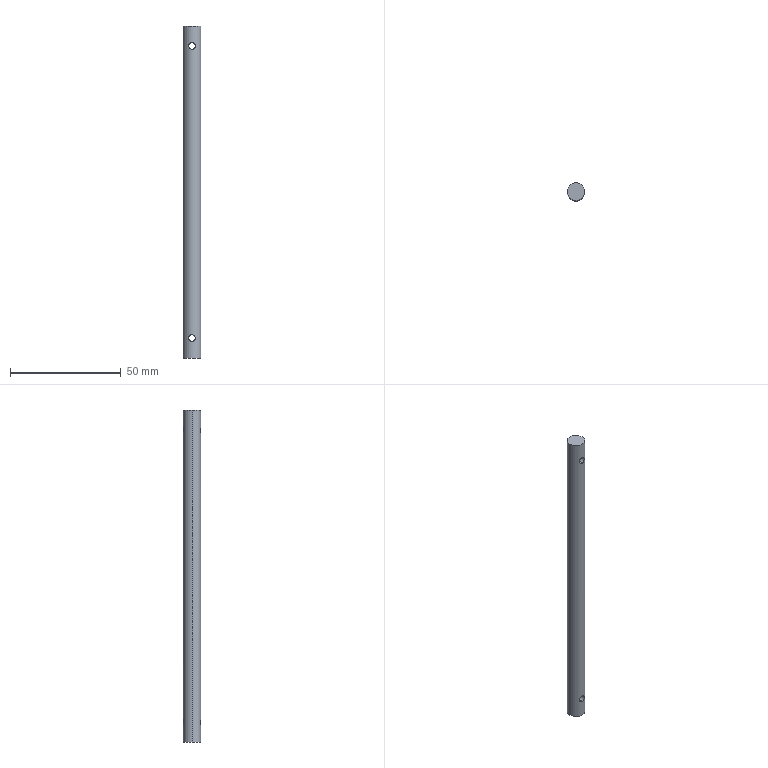Part | SolidWorks | features Extrusion 1, ICE 1 | 1 solid | 8 faces | box 8 x 8 x 150 mm | volume 7429 mm3 | cylinder 6 | plane 2 | commonest cylinder face diameters 3 x4 8 x2
STEP:
#1=CARTESIAN_POINT('',(0.,-4.,64.5));
#2=VERTEX_POINT('',#1);
#3=CARTESIAN_POINT('',(0.,-4.,67.5));
#4=VERTEX_POINT('',#3);
#5=CARTESIAN_POINT('',(0.,-4.,64.5));
#6=CARTESIAN_POINT('',(-0.1971,-4.,64.5));
#7=CARTESIAN_POINT('',(-0.396,-3.985,64.54));
#8=CARTESIAN_POINT('',(-0.6679,-3.945,64.653));
#9=CARTESIAN_POINT('',(-0.7555,-3.929,64.7));
#10=CARTESIAN_POINT('',(-0.917,-3.894,64.809));
#11=CARTESIAN_POINT('',(-0.9921,-3.876,64.871));
#12=CARTESIAN_POINT('',(-1.2,-3.818,65.079));
#13=CARTESIAN_POINT('',(-1.309,-3.78,65.242));
#14=CARTESIAN_POINT('',(-1.423,-3.739,65.515));
#15=CARTESIAN_POINT('',(-1.451,-3.727,65.608));
#16=CARTESIAN_POINT('',(-1.49,-3.712,65.801));
#17=CARTESIAN_POINT('',(-1.5,-3.708,65.902));
#18=CARTESIAN_POINT('',(-1.5,-3.708,66.198));
#19=CARTESIAN_POINT('',(-1.46,-3.725,66.397));
#20=CARTESIAN_POINT('',(-1.309,-3.781,66.758));
#21=CARTESIAN_POINT('',(-1.198,-3.819,66.923));
#22=CARTESIAN_POINT('',(-0.9915,-3.876,67.13));
#23=CARTESIAN_POINT('',(-0.9151,-3.895,67.193));
#24=CARTESIAN_POINT('',(-0.7535,-3.929,67.301));
#25=CARTESIAN_POINT('',(-0.6678,-3.945,67.347));
#26=CARTESIAN_POINT('',(-0.3945,-3.985,67.461));
#27=CARTESIAN_POINT('',(-0.2002,-4.,67.5));
#28=CARTESIAN_POINT('',(0.,-4.,67.5));
#29=B_SPLINE_CURVE_WITH_KNOTS('',3,(#5,#6,#7,#8,#9,#10,#11,#12,#13,#14,#15,#16,#17,#18,#19,#20,#21,#22,#23,#24,#25,#26,#27,#28),.UNSPECIFIED.,.F.,.F.,(4,2,2,2,2,2,2,2,2,2,2,4),(0.004733,0.005325,0.005621,0.005916,0.006508,0.006804,0.0071,0.007691,0.008283,0.008578,0.008874,0.009466),.UNSPECIFIED.);
#30=EDGE_CURVE('',#2,#4,#29,.T.);
#31=ORIENTED_EDGE('',*,*,#30,.F.);
#32=CARTESIAN_POINT('',(0.,4.,64.5));
#33=VERTEX_POINT('',#32);
#34=CARTESIAN_POINT('',(0.,-5.,64.5));
#35=DIRECTION('',(0.,1.,0.));
#36=VECTOR('',#35,1000.);
#37=LINE('',#34,#36);
#38=EDGE_CURVE('',#2,#33,#37,.T.);
#39=ORIENTED_EDGE('',*,*,#38,.T.);
#40=CARTESIAN_POINT('',(0.,4.,67.5));
#41=VERTEX_POINT('',#40);
#42=CARTESIAN_POINT('',(0.,4.,67.5));
#43=CARTESIAN_POINT('',(-0.1001,4.,67.5));
#44=CARTESIAN_POINT('',(-0.1983,3.996,67.49));
#45=CARTESIAN_POINT('',(-0.3914,3.982,67.451));
#46=CARTESIAN_POINT('',(-0.4871,3.971,67.422));
#47=CARTESIAN_POINT('',(-0.7591,3.932,67.309));
#48=CARTESIAN_POINT('',(-0.9243,3.894,67.197));
#49=CARTESIAN_POINT('',(-1.198,3.819,66.923));
#50=CARTESIAN_POINT('',(-1.309,3.78,66.757));
#51=CARTESIAN_POINT('',(-1.422,3.739,66.487));
#52=CARTESIAN_POINT('',(-1.451,3.727,66.392));
#53=CARTESIAN_POINT('',(-1.49,3.712,66.198));
#54=CARTESIAN_POINT('',(-1.5,3.708,66.1));
#55=CARTESIAN_POINT('',(-1.5,3.708,65.902));
#56=CARTESIAN_POINT('',(-1.49,3.712,65.802));
#57=CARTESIAN_POINT('',(-1.451,3.727,65.608));
#58=CARTESIAN_POINT('',(-1.423,3.739,65.514));
#59=CARTESIAN_POINT('',(-1.346,3.767,65.332));
#60=CARTESIAN_POINT('',(-1.3,3.783,65.246));
#61=CARTESIAN_POINT('',(-1.192,3.819,65.084));
#62=CARTESIAN_POINT('',(-1.129,3.838,65.008));
#63=CARTESIAN_POINT('',(-0.9914,3.876,64.87));
#64=CARTESIAN_POINT('',(-0.9166,3.894,64.809));
#65=CARTESIAN_POINT('',(-0.7545,3.929,64.7));
#66=CARTESIAN_POINT('',(-0.6669,3.945,64.653));
#67=CARTESIAN_POINT('',(-0.3963,3.984,64.54));
#68=CARTESIAN_POINT('',(-0.1972,4.,64.5));
#69=CARTESIAN_POINT('',(0.,4.,64.5));
#70=B_SPLINE_CURVE_WITH_KNOTS('',3,(#42,#43,#44,#45,#46,#47,#48,#49,#50,#51,#52,#53,#54,#55,#56,#57,#58,#59,#60,#61,#62,#63,#64,#65,#66,#67,#68,#69),.UNSPECIFIED.,.F.,.F.,(4,2,2,2,2,2,2,2,2,2,2,2,2,4),(0.,0.0002958,0.0005917,0.001183,0.001775,0.002071,0.002367,0.002663,0.002958,0.003254,0.00355,0.003846,0.004142,0.004733),.UNSPECIFIED.);
#71=EDGE_CURVE('',#41,#33,#70,.T.);
#72=ORIENTED_EDGE('',*,*,#71,.F.);
#73=CARTESIAN_POINT('',(0.,-5.,67.5));
#74=DIRECTION('',(0.,1.,0.));
#75=VECTOR('',#74,1000.);
#76=LINE('',#73,#75);
#77=EDGE_CURVE('',#4,#41,#76,.T.);
#78=ORIENTED_EDGE('',*,*,#77,.F.);
#79=EDGE_LOOP('',(#31,#39,#72,#78));
#80=FACE_OUTER_BOUND('',#79,.T.);
#81=CARTESIAN_POINT('',(0.,-5.,66.));
#82=DIRECTION('',(0.,1.,0.));
#83=DIRECTION('',(0.,0.,1.));
#84=AXIS2_PLACEMENT_3D('',#81,#82,#83);
#85=CYLINDRICAL_SURFACE('',#84,1.5);
#86=ADVANCED_FACE('',(#80),#85,.F.);
#87=CARTESIAN_POINT('',(0.,-4.,-67.5));
#88=VERTEX_POINT('',#87);
#89=CARTESIAN_POINT('',(0.,-4.,-64.5));
#90=VERTEX_POINT('',#89);
#91=CARTESIAN_POINT('',(0.,-4.,-67.5));
#92=CARTESIAN_POINT('',(-0.1971,-4.,-67.5));
#93=CARTESIAN_POINT('',(-0.396,-3.985,-67.46));
#94=CARTESIAN_POINT('',(-0.6679,-3.945,-67.347));
#95=CARTESIAN_POINT('',(-0.7555,-3.929,-67.3));
#96=CARTESIAN_POINT('',(-0.917,-3.894,-67.191));
#97=CARTESIAN_POINT('',(-0.9921,-3.876,-67.129));
#98=CARTESIAN_POINT('',(-1.2,-3.818,-66.921));
#99=CARTESIAN_POINT('',(-1.309,-3.78,-66.758));
#100=CARTESIAN_POINT('',(-1.423,-3.739,-66.485));
#101=CARTESIAN_POINT('',(-1.451,-3.727,-66.392));
#102=CARTESIAN_POINT('',(-1.49,-3.712,-66.199));
#103=CARTESIAN_POINT('',(-1.5,-3.708,-66.098));
#104=CARTESIAN_POINT('',(-1.5,-3.708,-65.802));
#105=CARTESIAN_POINT('',(-1.46,-3.725,-65.603));
#106=CARTESIAN_POINT('',(-1.309,-3.781,-65.242));
#107=CARTESIAN_POINT('',(-1.198,-3.819,-65.077));
#108=CARTESIAN_POINT('',(-0.9915,-3.876,-64.87));
#109=CARTESIAN_POINT('',(-0.9151,-3.895,-64.807));
#110=CARTESIAN_POINT('',(-0.7535,-3.929,-64.699));
#111=CARTESIAN_POINT('',(-0.6678,-3.945,-64.653));
#112=CARTESIAN_POINT('',(-0.3945,-3.985,-64.539));
#113=CARTESIAN_POINT('',(-0.2002,-4.,-64.5));
#114=CARTESIAN_POINT('',(0.,-4.,-64.5));
#115=B_SPLINE_CURVE_WITH_KNOTS('',3,(#91,#92,#93,#94,#95,#96,#97,#98,#99,#100,#101,#102,#103,#104,#105,#106,#107,#108,#109,#110,#111,#112,#113,#114),.UNSPECIFIED.,.F.,.F.,(4,2,2,2,2,2,2,2,2,2,2,4),(0.004733,0.005325,0.005621,0.005916,0.006508,0.006804,0.0071,0.007691,0.008283,0.008578,0.008874,0.009466),.UNSPECIFIED.);
#116=EDGE_CURVE('',#88,#90,#115,.T.);
#117=ORIENTED_EDGE('',*,*,#116,.F.);
#118=CARTESIAN_POINT('',(0.,4.,-67.5));
#119=VERTEX_POINT('',#118);
#120=CARTESIAN_POINT('',(0.,-5.,-67.5));
#121=DIRECTION('',(0.,1.,0.));
#122=VECTOR('',#121,1000.);
#123=LINE('',#120,#122);
#124=EDGE_CURVE('',#88,#119,#123,.T.);
#125=ORIENTED_EDGE('',*,*,#124,.T.);
#126=CARTESIAN_POINT('',(0.,4.,-64.5));
#127=VERTEX_POINT('',#126);
#128=CARTESIAN_POINT('',(0.,4.,-64.5));
#129=CARTESIAN_POINT('',(-0.1001,4.,-64.5));
#130=CARTESIAN_POINT('',(-0.1983,3.996,-64.51));
#131=CARTESIAN_POINT('',(-0.3914,3.982,-64.549));
#132=CARTESIAN_POINT('',(-0.4871,3.971,-64.578));
#133=CARTESIAN_POINT('',(-0.7591,3.932,-64.691));
#134=CARTESIAN_POINT('',(-0.9243,3.894,-64.803));
#135=CARTESIAN_POINT('',(-1.198,3.819,-65.077));
#136=CARTESIAN_POINT('',(-1.309,3.78,-65.243));
#137=CARTESIAN_POINT('',(-1.422,3.739,-65.513));
#138=CARTESIAN_POINT('',(-1.451,3.727,-65.608));
#139=CARTESIAN_POINT('',(-1.49,3.712,-65.802));
#140=CARTESIAN_POINT('',(-1.5,3.708,-65.9));
#141=CARTESIAN_POINT('',(-1.5,3.708,-66.098));
#142=CARTESIAN_POINT('',(-1.49,3.712,-66.198));
#143=CARTESIAN_POINT('',(-1.451,3.727,-66.392));
#144=CARTESIAN_POINT('',(-1.423,3.739,-66.486));
#145=CARTESIAN_POINT('',(-1.346,3.767,-66.668));
#146=CARTESIAN_POINT('',(-1.3,3.783,-66.754));
#147=CARTESIAN_POINT('',(-1.192,3.819,-66.916));
#148=CARTESIAN_POINT('',(-1.129,3.838,-66.992));
#149=CARTESIAN_POINT('',(-0.9914,3.876,-67.13));
#150=CARTESIAN_POINT('',(-0.9166,3.894,-67.191));
#151=CARTESIAN_POINT('',(-0.7545,3.929,-67.3));
#152=CARTESIAN_POINT('',(-0.6669,3.945,-67.347));
#153=CARTESIAN_POINT('',(-0.3963,3.984,-67.46));
#154=CARTESIAN_POINT('',(-0.1972,4.,-67.5));
#155=CARTESIAN_POINT('',(0.,4.,-67.5));
#156=B_SPLINE_CURVE_WITH_KNOTS('',3,(#128,#129,#130,#131,#132,#133,#134,#135,#136,#137,#138,#139,#140,#141,#142,#143,#144,#145,#146,#147,#148,#149,#150,#151,#152,#153,#154,#155),.UNSPECIFIED.,.F.,.F.,(4,2,2,2,2,2,2,2,2,2,2,2,2,4),(0.,0.0002958,0.0005917,0.001183,0.001775,0.002071,0.002367,0.002663,0.002958,0.003254,0.00355,0.003846,0.004142,0.004733),.UNSPECIFIED.);
#157=EDGE_CURVE('',#127,#119,#156,.T.);
#158=ORIENTED_EDGE('',*,*,#157,.F.);
#159=CARTESIAN_POINT('',(0.,-5.,-64.5));
#160=DIRECTION('',(0.,1.,0.));
#161=VECTOR('',#160,1000.);
#162=LINE('',#159,#161);
#163=EDGE_CURVE('',#90,#127,#162,.T.);
#164=ORIENTED_EDGE('',*,*,#163,.F.);
#165=EDGE_LOOP('',(#117,#125,#158,#164));
#166=FACE_OUTER_BOUND('',#165,.T.);
#167=CARTESIAN_POINT('',(0.,-5.,-66.));
#168=DIRECTION('',(0.,1.,0.));
#169=DIRECTION('',(0.,0.,1.));
#170=AXIS2_PLACEMENT_3D('',#167,#168,#169);
#171=CYLINDRICAL_SURFACE('',#170,1.5);
#172=ADVANCED_FACE('',(#166),#171,.F.);
#173=ORIENTED_EDGE('',*,*,#157,.T.);
#174=CARTESIAN_POINT('',(0.,4.,-67.5));
#175=CARTESIAN_POINT('',(0.1971,4.,-67.5));
#176=CARTESIAN_POINT('',(0.396,3.985,-67.46));
#177=CARTESIAN_POINT('',(0.6679,3.945,-67.347));
#178=CARTESIAN_POINT('',(0.7555,3.929,-67.3));
#179=CARTESIAN_POINT('',(0.917,3.894,-67.191));
#180=CARTESIAN_POINT('',(0.9921,3.876,-67.129));
#181=CARTESIAN_POINT('',(1.2,3.818,-66.921));
#182=CARTESIAN_POINT('',(1.309,3.78,-66.758));
#183=CARTESIAN_POINT('',(1.423,3.739,-66.485));
#184=CARTESIAN_POINT('',(1.451,3.727,-66.392));
#185=CARTESIAN_POINT('',(1.49,3.712,-66.199));
#186=CARTESIAN_POINT('',(1.5,3.708,-66.098));
#187=CARTESIAN_POINT('',(1.5,3.708,-65.802));
#188=CARTESIAN_POINT('',(1.46,3.725,-65.603));
#189=CARTESIAN_POINT('',(1.309,3.781,-65.242));
#190=CARTESIAN_POINT('',(1.198,3.819,-65.077));
#191=CARTESIAN_POINT('',(0.9915,3.876,-64.87));
#192=CARTESIAN_POINT('',(0.9151,3.895,-64.807));
#193=CARTESIAN_POINT('',(0.7535,3.929,-64.699));
#194=CARTESIAN_POINT('',(0.6678,3.945,-64.653));
#195=CARTESIAN_POINT('',(0.3945,3.985,-64.539));
#196=CARTESIAN_POINT('',(0.2002,4.,-64.5));
#197=CARTESIAN_POINT('',(0.,4.,-64.5));
#198=B_SPLINE_CURVE_WITH_KNOTS('',3,(#174,#175,#176,#177,#178,#179,#180,#181,#182,#183,#184,#185,#186,#187,#188,#189,#190,#191,#192,#193,#194,#195,#196,#197),.UNSPECIFIED.,.F.,.F.,(4,2,2,2,2,2,2,2,2,2,2,4),(0.004733,0.005325,0.005621,0.005916,0.006508,0.006804,0.0071,0.007691,0.008283,0.008578,0.008874,0.009466),.UNSPECIFIED.);
#199=EDGE_CURVE('',#119,#127,#198,.T.);
#200=ORIENTED_EDGE('',*,*,#199,.T.);
#201=EDGE_LOOP('',(#173,#200));
#202=FACE_BOUND('',#201,.T.);
#203=ORIENTED_EDGE('',*,*,#71,.T.);
#204=CARTESIAN_POINT('',(0.,4.,64.5));
#205=CARTESIAN_POINT('',(0.1971,4.,64.5));
#206=CARTESIAN_POINT('',(0.396,3.985,64.54));
#207=CARTESIAN_POINT('',(0.6679,3.945,64.653));
#208=CARTESIAN_POINT('',(0.7555,3.929,64.7));
#209=CARTESIAN_POINT('',(0.917,3.894,64.809));
#210=CARTESIAN_POINT('',(0.9921,3.876,64.871));
#211=CARTESIAN_POINT('',(1.2,3.818,65.079));
#212=CARTESIAN_POINT('',(1.309,3.78,65.242));
#213=CARTESIAN_POINT('',(1.423,3.739,65.515));
#214=CARTESIAN_POINT('',(1.451,3.727,65.608));
#215=CARTESIAN_POINT('',(1.49,3.712,65.801));
#216=CARTESIAN_POINT('',(1.5,3.708,65.902));
#217=CARTESIAN_POINT('',(1.5,3.708,66.198));
#218=CARTESIAN_POINT('',(1.46,3.725,66.397));
#219=CARTESIAN_POINT('',(1.309,3.781,66.758));
#220=CARTESIAN_POINT('',(1.198,3.819,66.923));
#221=CARTESIAN_POINT('',(0.9915,3.876,67.13));
#222=CARTESIAN_POINT('',(0.9151,3.895,67.193));
#223=CARTESIAN_POINT('',(0.7535,3.929,67.301));
#224=CARTESIAN_POINT('',(0.6678,3.945,67.347));
#225=CARTESIAN_POINT('',(0.3945,3.985,67.461));
#226=CARTESIAN_POINT('',(0.2002,4.,67.5));
#227=CARTESIAN_POINT('',(0.,4.,67.5));
#228=B_SPLINE_CURVE_WITH_KNOTS('',3,(#204,#205,#206,#207,#208,#209,#210,#211,#212,#213,#214,#215,#216,#217,#218,#219,#220,#221,#222,#223,#224,#225,#226,#227),.UNSPECIFIED.,.F.,.F.,(4,2,2,2,2,2,2,2,2,2,2,4),(0.004733,0.005325,0.005621,0.005916,0.006508,0.006804,0.0071,0.007691,0.008283,0.008578,0.008874,0.009466),.UNSPECIFIED.);
#229=EDGE_CURVE('',#33,#41,#228,.T.);
#230=ORIENTED_EDGE('',*,*,#229,.T.);
#231=EDGE_LOOP('',(#203,#230));
#232=FACE_BOUND('',#231,.T.);
#233=CARTESIAN_POINT('',(4.,0.,75.));
#234=VERTEX_POINT('',#233);
#235=CARTESIAN_POINT('',(-4.,0.,75.));
#236=VERTEX_POINT('',#235);
#237=CARTESIAN_POINT('',(0.,0.,75.));
#238=DIRECTION('',(0.,0.,1.));
#239=DIRECTION('',(1.,0.,0.));
#240=AXIS2_PLACEMENT_3D('',#237,#238,#239);
#241=CIRCLE('',#240,4.);
#242=EDGE_CURVE('',#234,#236,#241,.T.);
#243=ORIENTED_EDGE('',*,*,#242,.F.);
#244=CARTESIAN_POINT('',(4.,0.,-75.));
#245=VERTEX_POINT('',#244);
#246=CARTESIAN_POINT('',(4.,0.,75.));
#247=DIRECTION('',(0.,0.,-1.));
#248=VECTOR('',#247,1000.);
#249=LINE('',#246,#248);
#250=EDGE_CURVE('',#234,#245,#249,.T.);
#251=ORIENTED_EDGE('',*,*,#250,.T.);
#252=CARTESIAN_POINT('',(-4.,0.,-75.));
#253=VERTEX_POINT('',#252);
#254=CARTESIAN_POINT('',(0.,0.,-75.));
#255=DIRECTION('',(0.,0.,1.));
#256=DIRECTION('',(1.,0.,0.));
#257=AXIS2_PLACEMENT_3D('',#254,#255,#256);
#258=CIRCLE('',#257,4.);
#259=EDGE_CURVE('',#245,#253,#258,.T.);
#260=ORIENTED_EDGE('',*,*,#259,.T.);
#261=CARTESIAN_POINT('',(-4.,0.,75.));
#262=DIRECTION('',(0.,0.,-1.));
#263=VECTOR('',#262,1000.);
#264=LINE('',#261,#263);
#265=EDGE_CURVE('',#236,#253,#264,.T.);
#266=ORIENTED_EDGE('',*,*,#265,.F.);
#267=EDGE_LOOP('',(#243,#251,#260,#266));
#268=FACE_OUTER_BOUND('',#267,.T.);
#269=CARTESIAN_POINT('',(0.,0.,75.));
#270=DIRECTION('',(0.,0.,-1.));
#271=DIRECTION('',(-1.,0.,0.));
#272=AXIS2_PLACEMENT_3D('',#269,#270,#271);
#273=CYLINDRICAL_SURFACE('',#272,4.);
#274=ADVANCED_FACE('',(#202,#232,#268),#273,.T.);
#275=ORIENTED_EDGE('',*,*,#250,.F.);
#276=CARTESIAN_POINT('',(0.,0.,75.));
#277=DIRECTION('',(0.,0.,1.));
#278=DIRECTION('',(1.,0.,0.));
#279=AXIS2_PLACEMENT_3D('',#276,#277,#278);
#280=CIRCLE('',#279,4.);
#281=EDGE_CURVE('',#236,#234,#280,.T.);
#282=ORIENTED_EDGE('',*,*,#281,.F.);
#283=ORIENTED_EDGE('',*,*,#265,.T.);
#284=CARTESIAN_POINT('',(0.,0.,-75.));
#285=DIRECTION('',(0.,0.,1.));
#286=DIRECTION('',(1.,0.,0.));
#287=AXIS2_PLACEMENT_3D('',#284,#285,#286);
#288=CIRCLE('',#287,4.);
#289=EDGE_CURVE('',#253,#245,#288,.T.);
#290=ORIENTED_EDGE('',*,*,#289,.T.);
#291=EDGE_LOOP('',(#275,#282,#283,#290));
#292=FACE_OUTER_BOUND('',#291,.T.);
#293=CARTESIAN_POINT('',(0.,-4.,67.5));
#294=CARTESIAN_POINT('',(0.1001,-4.,67.5));
#295=CARTESIAN_POINT('',(0.1983,-3.996,67.49));
#296=CARTESIAN_POINT('',(0.3914,-3.982,67.451));
#297=CARTESIAN_POINT('',(0.4871,-3.971,67.422));
#298=CARTESIAN_POINT('',(0.7591,-3.932,67.309));
#299=CARTESIAN_POINT('',(0.9243,-3.894,67.197));
#300=CARTESIAN_POINT('',(1.198,-3.819,66.923));
#301=CARTESIAN_POINT('',(1.309,-3.78,66.757));
#302=CARTESIAN_POINT('',(1.422,-3.739,66.487));
#303=CARTESIAN_POINT('',(1.451,-3.727,66.392));
#304=CARTESIAN_POINT('',(1.49,-3.712,66.198));
#305=CARTESIAN_POINT('',(1.5,-3.708,66.1));
#306=CARTESIAN_POINT('',(1.5,-3.708,65.902));
#307=CARTESIAN_POINT('',(1.49,-3.712,65.802));
#308=CARTESIAN_POINT('',(1.451,-3.727,65.608));
#309=CARTESIAN_POINT('',(1.423,-3.739,65.514));
#310=CARTESIAN_POINT('',(1.346,-3.767,65.332));
#311=CARTESIAN_POINT('',(1.3,-3.783,65.246));
#312=CARTESIAN_POINT('',(1.192,-3.819,65.084));
#313=CARTESIAN_POINT('',(1.129,-3.838,65.008));
#314=CARTESIAN_POINT('',(0.9914,-3.876,64.87));
#315=CARTESIAN_POINT('',(0.9166,-3.894,64.809));
#316=CARTESIAN_POINT('',(0.7545,-3.929,64.7));
#317=CARTESIAN_POINT('',(0.6669,-3.945,64.653));
#318=CARTESIAN_POINT('',(0.3963,-3.984,64.54));
#319=CARTESIAN_POINT('',(0.1972,-4.,64.5));
#320=CARTESIAN_POINT('',(0.,-4.,64.5));
#321=B_SPLINE_CURVE_WITH_KNOTS('',3,(#293,#294,#295,#296,#297,#298,#299,#300,#301,#302,#303,#304,#305,#306,#307,#308,#309,#310,#311,#312,#313,#314,#315,#316,#317,#318,#319,#320),.UNSPECIFIED.,.F.,.F.,(4,2,2,2,2,2,2,2,2,2,2,2,2,4),(0.,0.0002958,0.0005917,0.001183,0.001775,0.002071,0.002367,0.002663,0.002958,0.003254,0.00355,0.003846,0.004142,0.004733),.UNSPECIFIED.);
#322=EDGE_CURVE('',#4,#2,#321,.T.);
#323=ORIENTED_EDGE('',*,*,#322,.T.);
#324=ORIENTED_EDGE('',*,*,#30,.T.);
#325=EDGE_LOOP('',(#323,#324));
#326=FACE_BOUND('',#325,.T.);
#327=CARTESIAN_POINT('',(0.,-4.,-64.5));
#328=CARTESIAN_POINT('',(0.1001,-4.,-64.5));
#329=CARTESIAN_POINT('',(0.1983,-3.996,-64.51));
#330=CARTESIAN_POINT('',(0.3914,-3.982,-64.549));
#331=CARTESIAN_POINT('',(0.4871,-3.971,-64.578));
#332=CARTESIAN_POINT('',(0.7591,-3.932,-64.691));
#333=CARTESIAN_POINT('',(0.9243,-3.894,-64.803));
#334=CARTESIAN_POINT('',(1.198,-3.819,-65.077));
#335=CARTESIAN_POINT('',(1.309,-3.78,-65.243));
#336=CARTESIAN_POINT('',(1.422,-3.739,-65.513));
#337=CARTESIAN_POINT('',(1.451,-3.727,-65.608));
#338=CARTESIAN_POINT('',(1.49,-3.712,-65.802));
#339=CARTESIAN_POINT('',(1.5,-3.708,-65.9));
#340=CARTESIAN_POINT('',(1.5,-3.708,-66.098));
#341=CARTESIAN_POINT('',(1.49,-3.712,-66.198));
#342=CARTESIAN_POINT('',(1.451,-3.727,-66.392));
#343=CARTESIAN_POINT('',(1.423,-3.739,-66.486));
#344=CARTESIAN_POINT('',(1.346,-3.767,-66.668));
#345=CARTESIAN_POINT('',(1.3,-3.783,-66.754));
#346=CARTESIAN_POINT('',(1.192,-3.819,-66.916));
#347=CARTESIAN_POINT('',(1.129,-3.838,-66.992));
#348=CARTESIAN_POINT('',(0.9914,-3.876,-67.13));
#349=CARTESIAN_POINT('',(0.9166,-3.894,-67.191));
#350=CARTESIAN_POINT('',(0.7545,-3.929,-67.3));
#351=CARTESIAN_POINT('',(0.6669,-3.945,-67.347));
#352=CARTESIAN_POINT('',(0.3963,-3.984,-67.46));
#353=CARTESIAN_POINT('',(0.1972,-4.,-67.5));
#354=CARTESIAN_POINT('',(0.,-4.,-67.5));
#355=B_SPLINE_CURVE_WITH_KNOTS('',3,(#327,#328,#329,#330,#331,#332,#333,#334,#335,#336,#337,#338,#339,#340,#341,#342,#343,#344,#345,#346,#347,#348,#349,#350,#351,#352,#353,#354),.UNSPECIFIED.,.F.,.F.,(4,2,2,2,2,2,2,2,2,2,2,2,2,4),(0.,0.0002958,0.0005917,0.001183,0.001775,0.002071,0.002367,0.002663,0.002958,0.003254,0.00355,0.003846,0.004142,0.004733),.UNSPECIFIED.);
#356=EDGE_CURVE('',#90,#88,#355,.T.);
#357=ORIENTED_EDGE('',*,*,#356,.T.);
#358=ORIENTED_EDGE('',*,*,#116,.T.);
#359=EDGE_LOOP('',(#357,#358));
#360=FACE_BOUND('',#359,.T.);
#361=CARTESIAN_POINT('',(0.,0.,75.));
#362=DIRECTION('',(0.,0.,-1.));
#363=DIRECTION('',(-1.,0.,0.));
#364=AXIS2_PLACEMENT_3D('',#361,#362,#363);
#365=CYLINDRICAL_SURFACE('',#364,4.);
#366=ADVANCED_FACE('',(#292,#326,#360),#365,.T.);
#367=ORIENTED_EDGE('',*,*,#281,.T.);
#368=ORIENTED_EDGE('',*,*,#242,.T.);
#369=EDGE_LOOP('',(#367,#368));
#370=FACE_OUTER_BOUND('',#369,.T.);
#371=CARTESIAN_POINT('',(0.,0.,75.));
#372=DIRECTION('',(0.,0.,1.));
#373=DIRECTION('',(1.,0.,0.));
#374=AXIS2_PLACEMENT_3D('',#371,#372,#373);
#375=PLANE('',#374);
#376=ADVANCED_FACE('',(#370),#375,.T.);
#377=ORIENTED_EDGE('',*,*,#289,.F.);
#378=ORIENTED_EDGE('',*,*,#259,.F.);
#379=EDGE_LOOP('',(#377,#378));
#380=FACE_OUTER_BOUND('',#379,.T.);
#381=CARTESIAN_POINT('',(0.,0.,-75.));
#382=DIRECTION('',(0.,0.,1.));
#383=DIRECTION('',(1.,0.,0.));
#384=AXIS2_PLACEMENT_3D('',#381,#382,#383);
#385=PLANE('',#384);
#386=ADVANCED_FACE('',(#380),#385,.F.);
#387=ORIENTED_EDGE('',*,*,#124,.F.);
#388=ORIENTED_EDGE('',*,*,#356,.F.);
#389=ORIENTED_EDGE('',*,*,#163,.T.);
#390=ORIENTED_EDGE('',*,*,#199,.F.);
#391=EDGE_LOOP('',(#387,#388,#389,#390));
#392=FACE_OUTER_BOUND('',#391,.T.);
#393=CARTESIAN_POINT('',(0.,-5.,-66.));
#394=DIRECTION('',(0.,1.,0.));
#395=DIRECTION('',(0.,0.,1.));
#396=AXIS2_PLACEMENT_3D('',#393,#394,#395);
#397=CYLINDRICAL_SURFACE('',#396,1.5);
#398=ADVANCED_FACE('',(#392),#397,.F.);
#399=ORIENTED_EDGE('',*,*,#38,.F.);
#400=ORIENTED_EDGE('',*,*,#322,.F.);
#401=ORIENTED_EDGE('',*,*,#77,.T.);
#402=ORIENTED_EDGE('',*,*,#229,.F.);
#403=EDGE_LOOP('',(#399,#400,#401,#402));
#404=FACE_OUTER_BOUND('',#403,.T.);
#405=CARTESIAN_POINT('',(0.,-5.,66.));
#406=DIRECTION('',(0.,1.,0.));
#407=DIRECTION('',(0.,0.,1.));
#408=AXIS2_PLACEMENT_3D('',#405,#406,#407);
#409=CYLINDRICAL_SURFACE('',#408,1.5);
#410=ADVANCED_FACE('',(#404),#409,.F.);
#411=CLOSED_SHELL('',(#86,#172,#274,#366,#376,#386,#398,#410));
#412=MANIFOLD_SOLID_BREP('',#411);
#413=CARTESIAN_POINT('',(0.,0.,0.));
#414=DIRECTION('',(0.,0.,1.));
#415=DIRECTION('',(1.,0.,0.));
#416=AXIS2_PLACEMENT_3D('',#413,#414,#415);
#417=(LENGTH_UNIT()NAMED_UNIT(*)SI_UNIT(.MILLI.,.METRE.));
#418=UNCERTAINTY_MEASURE_WITH_UNIT(LENGTH_MEASURE(0.00001),#417,'','');
#419=(NAMED_UNIT(*)PLANE_ANGLE_UNIT()SI_UNIT($,.RADIAN.));
#420=(NAMED_UNIT(*)SI_UNIT($,.STERADIAN.)SOLID_ANGLE_UNIT());
#421=(GEOMETRIC_REPRESENTATION_CONTEXT(3)GLOBAL_UNCERTAINTY_ASSIGNED_CONTEXT((#418))GLOBAL_UNIT_ASSIGNED_CONTEXT((#417,#419,#420))REPRESENTATION_CONTEXT('',''));
#422=ADVANCED_BREP_SHAPE_REPRESENTATION('',(#412,#416),#421);